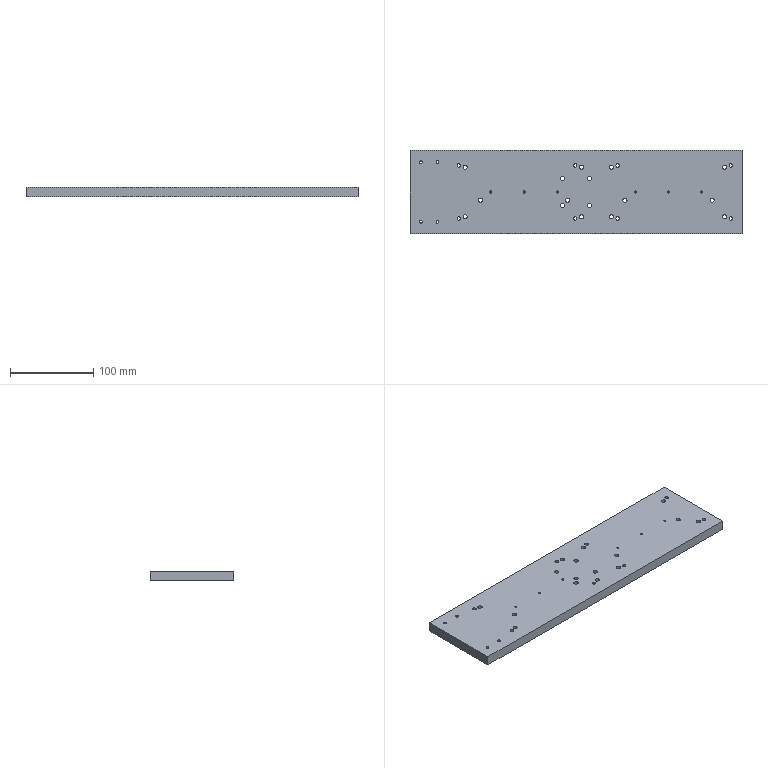Part | SolidWorks | features HoleWzd 4, Extrusion 1, ICE 1 | 1 solid | 74 faces | box 400 x 100 x 12 mm | volume 474136 mm3 | cylinder 68 | plane 6 | commonest cylinder face diameters 5 x32 4.2 x16 2.5 x12 3.3 x8